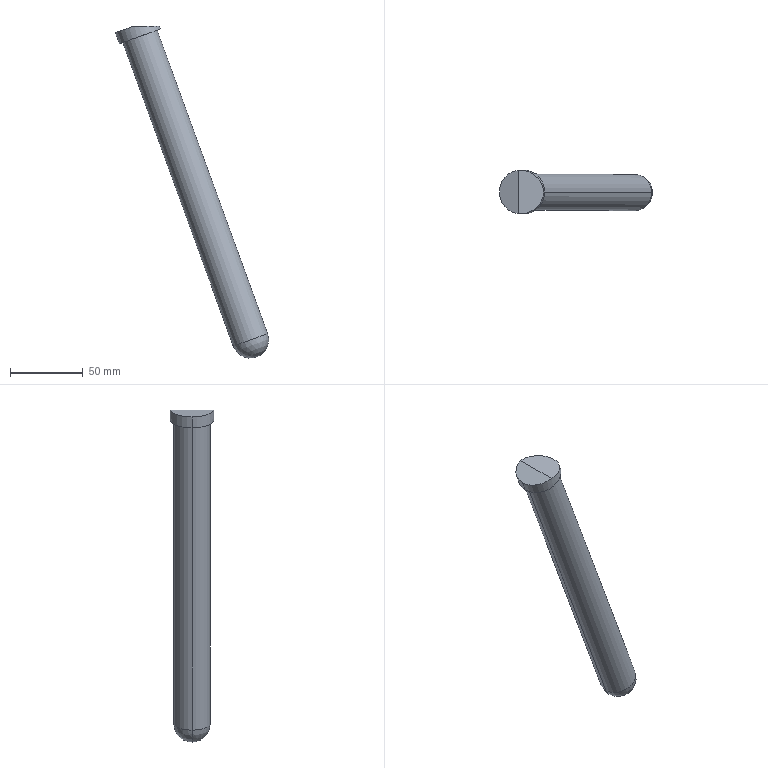Part | Creo | 1 solid | 9 faces | box 105.219 x 30.001 x 228.096 mm | volume 117675 mm3 | cylinder 4 | plane 3 | sphere 2 | commonest cylinder face diameters 25 x2 30 x2
STEP:
#1=CARTESIAN_POINT('',(253.855,112.995,47.033));
#2=VERTEX_POINT('',#1);
#3=CARTESIAN_POINT('',(225.664,112.995,36.772));
#4=VERTEX_POINT('',#3);
#5=CARTESIAN_POINT('',(239.76,112.995,41.903));
#6=DIRECTION('',(0.342,0.,-0.9397));
#7=DIRECTION('',(0.9397,0.,0.342));
#8=AXIS2_PLACEMENT_3D('',#5,#6,#7);
#9=CIRCLE('',#8,15.);
#10=EDGE_CURVE('',#2,#4,#9,.T.);
#11=ORIENTED_EDGE('',*,*,#10,.T.);
#12=CARTESIAN_POINT('',(222.928,112.995,44.29));
#13=VERTEX_POINT('',#12);
#14=CARTESIAN_POINT('',(222.928,112.995,44.29));
#15=DIRECTION('',(0.342,0.,-0.9397));
#16=VECTOR('',#15,8.);
#17=LINE('',#14,#16);
#18=EDGE_CURVE('',#13,#4,#17,.T.);
#19=ORIENTED_EDGE('',*,*,#18,.F.);
#20=CARTESIAN_POINT('',(235.869,98.046,49.));
#21=VERTEX_POINT('',#20);
#22=CARTESIAN_POINT('',(237.024,112.995,49.42));
#23=DIRECTION('',(-0.342,0.,0.9397));
#24=DIRECTION('',(-0.9397,0.,-0.342));
#25=AXIS2_PLACEMENT_3D('',#22,#23,#24);
#26=CIRCLE('',#25,15.);
#27=EDGE_CURVE('',#13,#21,#26,.T.);
#28=ORIENTED_EDGE('',*,*,#27,.T.);
#29=CARTESIAN_POINT('',(253.139,112.995,49.));
#30=VERTEX_POINT('',#29);
#31=CARTESIAN_POINT('',(253.139,112.995,49.));
#32=CARTESIAN_POINT('',(253.139,111.989,49.));
#33=CARTESIAN_POINT('',(252.929,110.011,49.));
#34=CARTESIAN_POINT('',(251.969,107.083,49.));
#35=CARTESIAN_POINT('',(250.376,104.378,49.));
#36=CARTESIAN_POINT('',(248.274,102.067,49.));
#37=CARTESIAN_POINT('',(245.627,100.141,49.));
#38=CARTESIAN_POINT('',(242.623,98.779,49.));
#39=CARTESIAN_POINT('',(239.334,98.019,49.));
#40=CARTESIAN_POINT('',(237.045,97.955,49.));
#41=CARTESIAN_POINT('',(235.869,98.046,49.));
#42=B_SPLINE_CURVE_WITH_KNOTS('',3,(#31,#32,#33,#34,#35,#36,#37,#38,#39,#40,#41),.UNSPECIFIED.,.F.,.F.,(4,1,1,1,1,1,1,1,4),(0.,0.125,0.25,0.375,0.5,0.625,0.75,0.875,1.),.UNSPECIFIED.);
#43=EDGE_CURVE('',#30,#21,#42,.T.);
#44=ORIENTED_EDGE('',*,*,#43,.F.);
#45=CARTESIAN_POINT('',(253.139,112.995,49.));
#46=DIRECTION('',(0.342,-0.000000016,-0.9397));
#47=VECTOR('',#46,2.093);
#48=LINE('',#45,#47);
#49=EDGE_CURVE('',#30,#2,#48,.T.);
#50=ORIENTED_EDGE('',*,*,#49,.T.);
#51=EDGE_LOOP('',(#11,#19,#28,#44,#50));
#52=FACE_OUTER_BOUND('',#51,.F.);
#53=CARTESIAN_POINT('',(232.329,112.995,62.317));
#54=DIRECTION('',(0.342,0.,-0.9397));
#55=DIRECTION('',(0.9397,0.,0.342));
#56=AXIS2_PLACEMENT_3D('',#53,#54,#55);
#57=CYLINDRICAL_SURFACE('',#56,15.);
#58=ADVANCED_FACE('',(#52),#57,.T.);
#59=CARTESIAN_POINT('',(239.76,112.995,41.903));
#60=DIRECTION('',(0.342,0.,-0.9397));
#61=DIRECTION('',(-0.9397,0.,-0.342));
#62=AXIS2_PLACEMENT_3D('',#59,#60,#61);
#63=CIRCLE('',#62,15.);
#64=EDGE_CURVE('',#4,#2,#63,.T.);
#65=ORIENTED_EDGE('',*,*,#64,.F.);
#66=ORIENTED_EDGE('',*,*,#10,.F.);
#67=EDGE_LOOP('',(#65,#66));
#68=FACE_OUTER_BOUND('',#67,.F.);
#69=CARTESIAN_POINT('',(228.014,112.995,37.627));
#70=VERTEX_POINT('',#69);
#71=CARTESIAN_POINT('',(251.506,112.995,46.178));
#72=VERTEX_POINT('',#71);
#73=CARTESIAN_POINT('',(239.76,112.995,41.903));
#74=DIRECTION('',(-0.342,0.,0.9397));
#75=DIRECTION('',(-0.9397,0.,-0.342));
#76=AXIS2_PLACEMENT_3D('',#73,#74,#75);
#77=CIRCLE('',#76,12.5);
#78=EDGE_CURVE('',#70,#72,#77,.T.);
#79=ORIENTED_EDGE('',*,*,#78,.F.);
#80=CARTESIAN_POINT('',(239.76,112.995,41.903));
#81=DIRECTION('',(-0.342,0.,0.9397));
#82=DIRECTION('',(0.9397,0.,0.342));
#83=AXIS2_PLACEMENT_3D('',#80,#81,#82);
#84=CIRCLE('',#83,12.5);
#85=EDGE_CURVE('',#72,#70,#84,.T.);
#86=ORIENTED_EDGE('',*,*,#85,.F.);
#87=EDGE_LOOP('',(#79,#86));
#88=FACE_BOUND('',#87,.F.);
#89=CARTESIAN_POINT('',(239.76,112.995,41.903));
#90=DIRECTION('',(0.342,0.,-0.9397));
#91=DIRECTION('',(0.9397,0.,0.342));
#92=AXIS2_PLACEMENT_3D('',#89,#90,#91);
#93=PLANE('',#92);
#94=ADVANCED_FACE('',(#68,#88),#93,.T.);
#95=CARTESIAN_POINT('',(327.393,112.995,-162.321));
#96=VERTEX_POINT('',#95);
#97=CARTESIAN_POINT('',(303.901,112.995,-170.872));
#98=VERTEX_POINT('',#97);
#99=CARTESIAN_POINT('',(315.647,112.995,-166.596));
#100=DIRECTION('',(0.342,0.,-0.9397));
#101=DIRECTION('',(0.9397,0.,0.342));
#102=AXIS2_PLACEMENT_3D('',#99,#100,#101);
#103=CIRCLE('',#102,12.5);
#104=EDGE_CURVE('',#96,#98,#103,.T.);
#105=ORIENTED_EDGE('',*,*,#104,.T.);
#106=CARTESIAN_POINT('',(228.014,112.995,37.627));
#107=DIRECTION('',(0.342,0.,-0.9397));
#108=VECTOR('',#107,221.88);
#109=LINE('',#106,#108);
#110=EDGE_CURVE('',#70,#98,#109,.T.);
#111=ORIENTED_EDGE('',*,*,#110,.F.);
#112=ORIENTED_EDGE('',*,*,#78,.T.);
#113=CARTESIAN_POINT('',(251.506,112.995,46.178));
#114=DIRECTION('',(0.342,0.,-0.9397));
#115=VECTOR('',#114,221.88);
#116=LINE('',#113,#115);
#117=EDGE_CURVE('',#72,#96,#116,.T.);
#118=ORIENTED_EDGE('',*,*,#117,.T.);
#119=EDGE_LOOP('',(#105,#111,#112,#118));
#120=FACE_OUTER_BOUND('',#119,.F.);
#121=CARTESIAN_POINT('',(217.923,112.995,101.897));
#122=DIRECTION('',(0.342,0.,-0.9397));
#123=DIRECTION('',(0.9397,0.,0.342));
#124=AXIS2_PLACEMENT_3D('',#121,#122,#123);
#125=CYLINDRICAL_SURFACE('',#124,12.5);
#126=ADVANCED_FACE('',(#120),#125,.T.);
#127=ORIENTED_EDGE('',*,*,#104,.F.);
#128=CARTESIAN_POINT('',(319.922,112.995,-178.343));
#129=VERTEX_POINT('',#128);
#130=CARTESIAN_POINT('',(315.647,112.995,-166.596));
#131=DIRECTION('',(0.,1.,0.));
#132=DIRECTION('',(0.9397,0.,0.342));
#133=AXIS2_PLACEMENT_3D('',#130,#131,#132);
#134=CIRCLE('',#133,12.5);
#135=EDGE_CURVE('',#96,#129,#134,.T.);
#136=ORIENTED_EDGE('',*,*,#135,.T.);
#137=CARTESIAN_POINT('',(315.647,112.995,-166.596));
#138=DIRECTION('',(0.,-1.,0.));
#139=DIRECTION('',(-0.9397,0.,-0.342));
#140=AXIS2_PLACEMENT_3D('',#137,#138,#139);
#141=CIRCLE('',#140,12.5);
#142=EDGE_CURVE('',#98,#129,#141,.T.);
#143=ORIENTED_EDGE('',*,*,#142,.F.);
#144=EDGE_LOOP('',(#127,#136,#143));
#145=FACE_OUTER_BOUND('',#144,.F.);
#146=CARTESIAN_POINT('',(315.647,112.995,-166.596));
#147=DIRECTION('',(0.342,0.,-0.9397));
#148=DIRECTION('',(0.9397,0.,0.342));
#149=AXIS2_PLACEMENT_3D('',#146,#147,#148);
#150=SPHERICAL_SURFACE('',#149,12.5);
#151=ADVANCED_FACE('',(#145),#150,.T.);
#152=CARTESIAN_POINT('',(315.647,112.995,-166.596));
#153=DIRECTION('',(0.342,0.,-0.9397));
#154=DIRECTION('',(-0.9397,0.,-0.342));
#155=AXIS2_PLACEMENT_3D('',#152,#153,#154);
#156=CIRCLE('',#155,12.5);
#157=EDGE_CURVE('',#98,#96,#156,.T.);
#158=ORIENTED_EDGE('',*,*,#157,.F.);
#159=ORIENTED_EDGE('',*,*,#142,.T.);
#160=ORIENTED_EDGE('',*,*,#135,.F.);
#161=EDGE_LOOP('',(#158,#159,#160));
#162=FACE_OUTER_BOUND('',#161,.F.);
#163=CARTESIAN_POINT('',(315.647,112.995,-166.596));
#164=DIRECTION('',(0.342,0.,-0.9397));
#165=DIRECTION('',(0.9397,0.,0.342));
#166=AXIS2_PLACEMENT_3D('',#163,#164,#165);
#167=SPHERICAL_SURFACE('',#166,12.5);
#168=ADVANCED_FACE('',(#162),#167,.T.);
#169=ORIENTED_EDGE('',*,*,#157,.T.);
#170=ORIENTED_EDGE('',*,*,#117,.F.);
#171=ORIENTED_EDGE('',*,*,#85,.T.);
#172=ORIENTED_EDGE('',*,*,#110,.T.);
#173=EDGE_LOOP('',(#169,#170,#171,#172));
#174=FACE_OUTER_BOUND('',#173,.F.);
#175=CARTESIAN_POINT('',(217.923,112.995,101.897));
#176=DIRECTION('',(0.342,0.,-0.9397));
#177=DIRECTION('',(0.9397,0.,0.342));
#178=AXIS2_PLACEMENT_3D('',#175,#176,#177);
#179=CYLINDRICAL_SURFACE('',#178,12.5);
#180=ADVANCED_FACE('',(#174),#179,.T.);
#181=ORIENTED_EDGE('',*,*,#64,.T.);
#182=ORIENTED_EDGE('',*,*,#49,.F.);
#183=CARTESIAN_POINT('',(235.869,127.945,49.));
#184=VERTEX_POINT('',#183);
#185=CARTESIAN_POINT('',(253.139,112.995,49.));
#186=CARTESIAN_POINT('',(253.139,113.903,49.));
#187=CARTESIAN_POINT('',(252.966,115.681,49.));
#188=CARTESIAN_POINT('',(252.216,118.254,49.));
#189=CARTESIAN_POINT('',(250.989,120.675,49.));
#190=CARTESIAN_POINT('',(249.288,122.894,49.));
#191=CARTESIAN_POINT('',(247.169,124.8,49.));
#192=CARTESIAN_POINT('',(244.702,126.321,49.));
#193=CARTESIAN_POINT('',(241.929,127.41,49.));
#194=CARTESIAN_POINT('',(238.939,127.995,49.));
#195=CARTESIAN_POINT('',(236.905,128.025,49.));
#196=CARTESIAN_POINT('',(235.869,127.945,49.));
#197=B_SPLINE_CURVE_WITH_KNOTS('',3,(#185,#186,#187,#188,#189,#190,#191,#192,#193,#194,#195,#196),.UNSPECIFIED.,.F.,.F.,(4,1,1,1,1,1,1,1,1,4),(0.,0.1111,0.2222,0.3333,0.4444,0.5556,0.6667,0.7778,0.8889,1.),.UNSPECIFIED.);
#198=EDGE_CURVE('',#30,#184,#197,.T.);
#199=ORIENTED_EDGE('',*,*,#198,.T.);
#200=CARTESIAN_POINT('',(237.024,112.995,49.42));
#201=DIRECTION('',(-0.342,0.,0.9397));
#202=DIRECTION('',(-0.07697,0.9966,-0.02801));
#203=AXIS2_PLACEMENT_3D('',#200,#201,#202);
#204=CIRCLE('',#203,15.);
#205=EDGE_CURVE('',#184,#13,#204,.T.);
#206=ORIENTED_EDGE('',*,*,#205,.T.);
#207=ORIENTED_EDGE('',*,*,#18,.T.);
#208=EDGE_LOOP('',(#181,#182,#199,#206,#207));
#209=FACE_OUTER_BOUND('',#208,.F.);
#210=CARTESIAN_POINT('',(232.329,112.995,62.317));
#211=DIRECTION('',(0.342,0.,-0.9397));
#212=DIRECTION('',(0.9397,0.,0.342));
#213=AXIS2_PLACEMENT_3D('',#210,#211,#212);
#214=CYLINDRICAL_SURFACE('',#213,15.);
#215=ADVANCED_FACE('',(#209),#214,.T.);
#216=ORIENTED_EDGE('',*,*,#198,.F.);
#217=ORIENTED_EDGE('',*,*,#43,.T.);
#218=CARTESIAN_POINT('',(235.869,98.046,49.));
#219=DIRECTION('',(0.,1.,0.));
#220=VECTOR('',#219,29.899);
#221=LINE('',#218,#220);
#222=EDGE_CURVE('',#21,#184,#221,.T.);
#223=ORIENTED_EDGE('',*,*,#222,.T.);
#224=EDGE_LOOP('',(#216,#217,#223));
#225=FACE_OUTER_BOUND('',#224,.F.);
#226=CARTESIAN_POINT('',(242.333,252.939,49.));
#227=DIRECTION('',(0.,0.,1.));
#228=DIRECTION('',(0.,-1.,0.));
#229=AXIS2_PLACEMENT_3D('',#226,#227,#228);
#230=PLANE('',#229);
#231=ADVANCED_FACE('',(#225),#230,.T.);
#232=ORIENTED_EDGE('',*,*,#27,.F.);
#233=ORIENTED_EDGE('',*,*,#205,.F.);
#234=ORIENTED_EDGE('',*,*,#222,.F.);
#235=EDGE_LOOP('',(#232,#233,#234));
#236=FACE_OUTER_BOUND('',#235,.F.);
#237=CARTESIAN_POINT('',(237.024,112.995,49.42));
#238=DIRECTION('',(0.342,0.,-0.9397));
#239=DIRECTION('',(0.9397,0.,0.342));
#240=AXIS2_PLACEMENT_3D('',#237,#238,#239);
#241=PLANE('',#240);
#242=ADVANCED_FACE('',(#236),#241,.F.);
#243=CLOSED_SHELL('',(#58,#94,#126,#151,#168,#180,#215,#231,#242));
#244=MANIFOLD_SOLID_BREP('',#243);
#245=(LENGTH_UNIT()NAMED_UNIT(*)SI_UNIT(.MILLI.,.METRE.));
#246=UNCERTAINTY_MEASURE_WITH_UNIT(LENGTH_MEASURE(0.0258),#245,'','');
#247=(NAMED_UNIT(*)PLANE_ANGLE_UNIT()SI_UNIT($,.RADIAN.));
#248=PLANE_ANGLE_MEASURE_WITH_UNIT(PLANE_ANGLE_MEASURE(0.01745),#247);
#249=(CONVERSION_BASED_UNIT('DEGREE',#248)NAMED_UNIT(*)PLANE_ANGLE_UNIT());
#250=(NAMED_UNIT(*)SI_UNIT($,.STERADIAN.)SOLID_ANGLE_UNIT());
#251=(GEOMETRIC_REPRESENTATION_CONTEXT(3)GLOBAL_UNCERTAINTY_ASSIGNED_CONTEXT((#246))GLOBAL_UNIT_ASSIGNED_CONTEXT((#245,#249,#250))REPRESENTATION_CONTEXT('',''));
#252=ADVANCED_BREP_SHAPE_REPRESENTATION('',(#244),#251);